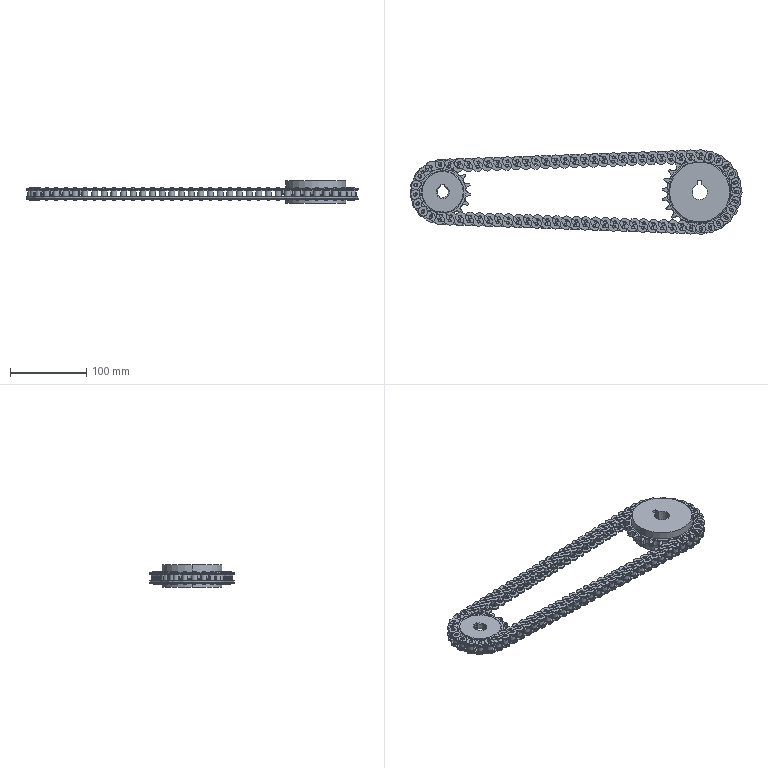Part | SolidWorks | features ReferencePattern 73, Belt 1, LocalChainPattern 1 | 224 solids | 4905 faces | volume 364523 mm3 | cylinder 3233 | plane 982 | cone 598 | torus 92 | commonest cylinder face diameters 3.98 x1184 12.07 x444 12.33 x444 7.92 x296 43.376 x296 55.348 x296